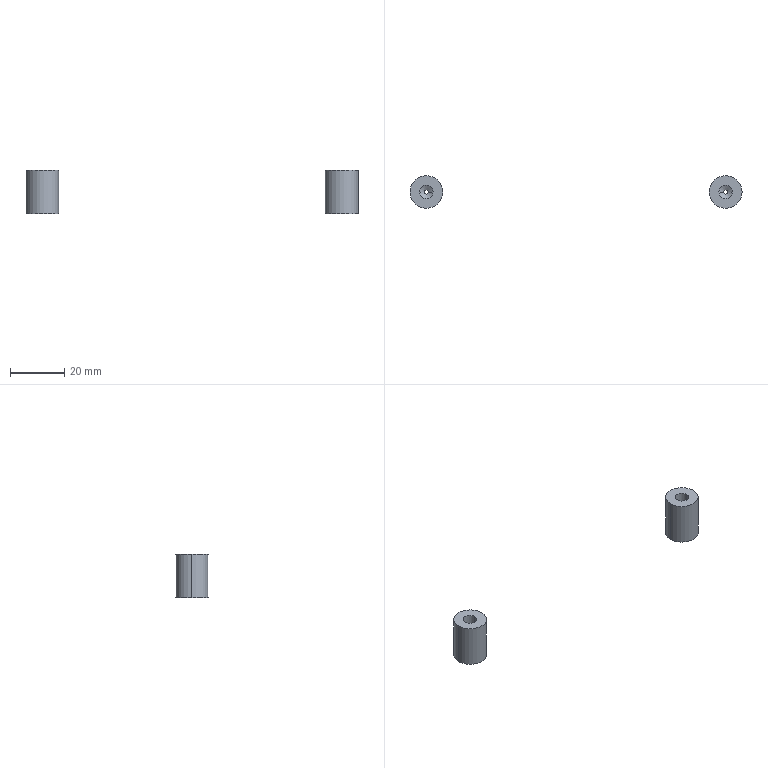Part | SolidWorks | features BaseBody 2 | 2 solids | 16 faces | box 122 x 12 x 16 mm | volume 3011 mm3 | cylinder 8 | cone 4 | plane 4 | commonest cylinder face diameters 5 x4 12 x4
STEP:
#1=CARTESIAN_POINT('',(-6.,0.,16.));
#2=VERTEX_POINT('',#1);
#3=CARTESIAN_POINT('',(6.,0.,16.));
#4=VERTEX_POINT('',#3);
#5=CARTESIAN_POINT('',(0.,0.,16.));
#6=DIRECTION('',(0.,0.,-1.));
#7=DIRECTION('',(-1.,0.,0.));
#8=AXIS2_PLACEMENT_3D('',#5,#6,#7);
#9=CIRCLE('',#8,6.);
#10=EDGE_CURVE('',#2,#4,#9,.T.);
#11=ORIENTED_EDGE('',*,*,#10,.T.);
#12=CARTESIAN_POINT('',(6.,0.,0.));
#13=VERTEX_POINT('',#12);
#14=CARTESIAN_POINT('',(6.,0.,16.));
#15=DIRECTION('',(0.,0.,-1.));
#16=VECTOR('',#15,1000.);
#17=LINE('',#14,#16);
#18=EDGE_CURVE('',#4,#13,#17,.T.);
#19=ORIENTED_EDGE('',*,*,#18,.T.);
#20=CARTESIAN_POINT('',(-6.,0.,0.));
#21=VERTEX_POINT('',#20);
#22=CARTESIAN_POINT('',(0.,0.,0.));
#23=DIRECTION('',(0.,0.,1.));
#24=DIRECTION('',(-1.,0.,0.));
#25=AXIS2_PLACEMENT_3D('',#22,#23,#24);
#26=CIRCLE('',#25,6.);
#27=EDGE_CURVE('',#13,#21,#26,.T.);
#28=ORIENTED_EDGE('',*,*,#27,.T.);
#29=CARTESIAN_POINT('',(-6.,0.,16.));
#30=DIRECTION('',(0.,0.,-1.));
#31=VECTOR('',#30,1000.);
#32=LINE('',#29,#31);
#33=EDGE_CURVE('',#2,#21,#32,.T.);
#34=ORIENTED_EDGE('',*,*,#33,.F.);
#35=EDGE_LOOP('',(#11,#19,#28,#34));
#36=FACE_OUTER_BOUND('',#35,.T.);
#37=CARTESIAN_POINT('',(0.,0.,16.));
#38=DIRECTION('',(0.,0.,-1.));
#39=DIRECTION('',(-1.,0.,0.));
#40=AXIS2_PLACEMENT_3D('',#37,#38,#39);
#41=CYLINDRICAL_SURFACE('',#40,6.);
#42=ADVANCED_FACE('',(#36),#41,.T.);
#43=CARTESIAN_POINT('',(0.8357,0.,0.));
#44=VERTEX_POINT('',#43);
#45=CARTESIAN_POINT('',(-0.8357,0.,0.));
#46=VERTEX_POINT('',#45);
#47=CARTESIAN_POINT('',(0.,0.,0.));
#48=DIRECTION('',(0.,0.,-1.));
#49=DIRECTION('',(1.,0.,0.));
#50=AXIS2_PLACEMENT_3D('',#47,#48,#49);
#51=CIRCLE('',#50,0.8357);
#52=EDGE_CURVE('',#44,#46,#51,.T.);
#53=ORIENTED_EDGE('',*,*,#52,.T.);
#54=CARTESIAN_POINT('',(-2.5,0.,1.));
#55=VERTEX_POINT('',#54);
#56=CARTESIAN_POINT('',(-2.5,0.,1.));
#57=DIRECTION('',(-0.8572,0.,0.515));
#58=VECTOR('',#57,1000.);
#59=LINE('',#56,#58);
#60=EDGE_CURVE('',#46,#55,#59,.T.);
#61=ORIENTED_EDGE('',*,*,#60,.T.);
#62=CARTESIAN_POINT('',(2.5,0.,1.));
#63=VERTEX_POINT('',#62);
#64=CARTESIAN_POINT('',(0.,0.,1.));
#65=DIRECTION('',(0.,0.,-1.));
#66=DIRECTION('',(1.,0.,0.));
#67=AXIS2_PLACEMENT_3D('',#64,#65,#66);
#68=CIRCLE('',#67,2.5);
#69=EDGE_CURVE('',#63,#55,#68,.T.);
#70=ORIENTED_EDGE('',*,*,#69,.F.);
#71=CARTESIAN_POINT('',(2.5,0.,1.));
#72=DIRECTION('',(0.8572,0.,0.515));
#73=VECTOR('',#72,1000.);
#74=LINE('',#71,#73);
#75=EDGE_CURVE('',#44,#63,#74,.T.);
#76=ORIENTED_EDGE('',*,*,#75,.F.);
#77=EDGE_LOOP('',(#53,#61,#70,#76));
#78=FACE_OUTER_BOUND('',#77,.T.);
#79=CARTESIAN_POINT('',(0.,0.,1.));
#80=DIRECTION('',(0.,0.,1.));
#81=DIRECTION('',(1.,0.,0.));
#82=AXIS2_PLACEMENT_3D('',#79,#80,#81);
#83=CONICAL_SURFACE('',#82,2.5,1.03);
#84=ADVANCED_FACE('',(#78),#83,.F.);
#85=ORIENTED_EDGE('',*,*,#69,.T.);
#86=CARTESIAN_POINT('',(-2.5,0.,16.));
#87=VERTEX_POINT('',#86);
#88=CARTESIAN_POINT('',(-2.5,0.,16.));
#89=DIRECTION('',(0.,0.,1.));
#90=VECTOR('',#89,1000.);
#91=LINE('',#88,#90);
#92=EDGE_CURVE('',#55,#87,#91,.T.);
#93=ORIENTED_EDGE('',*,*,#92,.T.);
#94=CARTESIAN_POINT('',(2.5,0.,16.));
#95=VERTEX_POINT('',#94);
#96=CARTESIAN_POINT('',(0.,0.,16.));
#97=DIRECTION('',(0.,0.,-1.));
#98=DIRECTION('',(1.,0.,0.));
#99=AXIS2_PLACEMENT_3D('',#96,#97,#98);
#100=CIRCLE('',#99,2.5);
#101=EDGE_CURVE('',#95,#87,#100,.T.);
#102=ORIENTED_EDGE('',*,*,#101,.F.);
#103=CARTESIAN_POINT('',(2.5,0.,16.));
#104=DIRECTION('',(0.,0.,1.));
#105=VECTOR('',#104,1000.);
#106=LINE('',#103,#105);
#107=EDGE_CURVE('',#63,#95,#106,.T.);
#108=ORIENTED_EDGE('',*,*,#107,.F.);
#109=EDGE_LOOP('',(#85,#93,#102,#108));
#110=FACE_OUTER_BOUND('',#109,.T.);
#111=CARTESIAN_POINT('',(0.,0.,16.));
#112=DIRECTION('',(0.,0.,1.));
#113=DIRECTION('',(1.,0.,0.));
#114=AXIS2_PLACEMENT_3D('',#111,#112,#113);
#115=CYLINDRICAL_SURFACE('',#114,2.5);
#116=ADVANCED_FACE('',(#110),#115,.F.);
#117=ORIENTED_EDGE('',*,*,#18,.F.);
#118=CARTESIAN_POINT('',(0.,0.,16.));
#119=DIRECTION('',(0.,0.,-1.));
#120=DIRECTION('',(-1.,0.,0.));
#121=AXIS2_PLACEMENT_3D('',#118,#119,#120);
#122=CIRCLE('',#121,6.);
#123=EDGE_CURVE('',#4,#2,#122,.T.);
#124=ORIENTED_EDGE('',*,*,#123,.T.);
#125=ORIENTED_EDGE('',*,*,#33,.T.);
#126=CARTESIAN_POINT('',(0.,0.,0.));
#127=DIRECTION('',(0.,0.,1.));
#128=DIRECTION('',(-1.,0.,0.));
#129=AXIS2_PLACEMENT_3D('',#126,#127,#128);
#130=CIRCLE('',#129,6.);
#131=EDGE_CURVE('',#21,#13,#130,.T.);
#132=ORIENTED_EDGE('',*,*,#131,.T.);
#133=EDGE_LOOP('',(#117,#124,#125,#132));
#134=FACE_OUTER_BOUND('',#133,.T.);
#135=CARTESIAN_POINT('',(0.,0.,16.));
#136=DIRECTION('',(0.,0.,-1.));
#137=DIRECTION('',(-1.,0.,0.));
#138=AXIS2_PLACEMENT_3D('',#135,#136,#137);
#139=CYLINDRICAL_SURFACE('',#138,6.);
#140=ADVANCED_FACE('',(#134),#139,.T.);
#141=ORIENTED_EDGE('',*,*,#131,.F.);
#142=ORIENTED_EDGE('',*,*,#27,.F.);
#143=EDGE_LOOP('',(#141,#142));
#144=FACE_OUTER_BOUND('',#143,.T.);
#145=ORIENTED_EDGE('',*,*,#52,.F.);
#146=CARTESIAN_POINT('',(0.,0.,0.));
#147=DIRECTION('',(0.,0.,-1.));
#148=DIRECTION('',(1.,0.,0.));
#149=AXIS2_PLACEMENT_3D('',#146,#147,#148);
#150=CIRCLE('',#149,0.8357);
#151=EDGE_CURVE('',#46,#44,#150,.T.);
#152=ORIENTED_EDGE('',*,*,#151,.F.);
#153=EDGE_LOOP('',(#145,#152));
#154=FACE_BOUND('',#153,.T.);
#155=CARTESIAN_POINT('',(0.,0.,0.));
#156=DIRECTION('',(0.,0.,1.));
#157=DIRECTION('',(1.,0.,0.));
#158=AXIS2_PLACEMENT_3D('',#155,#156,#157);
#159=PLANE('',#158);
#160=ADVANCED_FACE('',(#144,#154),#159,.F.);
#161=ORIENTED_EDGE('',*,*,#10,.F.);
#162=ORIENTED_EDGE('',*,*,#123,.F.);
#163=EDGE_LOOP('',(#161,#162));
#164=FACE_OUTER_BOUND('',#163,.T.);
#165=ORIENTED_EDGE('',*,*,#101,.T.);
#166=CARTESIAN_POINT('',(0.,0.,16.));
#167=DIRECTION('',(0.,0.,-1.));
#168=DIRECTION('',(1.,0.,0.));
#169=AXIS2_PLACEMENT_3D('',#166,#167,#168);
#170=CIRCLE('',#169,2.5);
#171=EDGE_CURVE('',#87,#95,#170,.T.);
#172=ORIENTED_EDGE('',*,*,#171,.T.);
#173=EDGE_LOOP('',(#165,#172));
#174=FACE_BOUND('',#173,.T.);
#175=CARTESIAN_POINT('',(0.,0.,16.));
#176=DIRECTION('',(0.,0.,1.));
#177=DIRECTION('',(1.,0.,0.));
#178=AXIS2_PLACEMENT_3D('',#175,#176,#177);
#179=PLANE('',#178);
#180=ADVANCED_FACE('',(#164,#174),#179,.T.);
#181=ORIENTED_EDGE('',*,*,#60,.F.);
#182=ORIENTED_EDGE('',*,*,#151,.T.);
#183=ORIENTED_EDGE('',*,*,#75,.T.);
#184=CARTESIAN_POINT('',(0.,0.,1.));
#185=DIRECTION('',(0.,0.,-1.));
#186=DIRECTION('',(1.,0.,0.));
#187=AXIS2_PLACEMENT_3D('',#184,#185,#186);
#188=CIRCLE('',#187,2.5);
#189=EDGE_CURVE('',#55,#63,#188,.T.);
#190=ORIENTED_EDGE('',*,*,#189,.F.);
#191=EDGE_LOOP('',(#181,#182,#183,#190));
#192=FACE_OUTER_BOUND('',#191,.T.);
#193=CARTESIAN_POINT('',(0.,0.,1.));
#194=DIRECTION('',(0.,0.,1.));
#195=DIRECTION('',(1.,0.,0.));
#196=AXIS2_PLACEMENT_3D('',#193,#194,#195);
#197=CONICAL_SURFACE('',#196,2.5,1.03);
#198=ADVANCED_FACE('',(#192),#197,.F.);
#199=ORIENTED_EDGE('',*,*,#92,.F.);
#200=ORIENTED_EDGE('',*,*,#189,.T.);
#201=ORIENTED_EDGE('',*,*,#107,.T.);
#202=ORIENTED_EDGE('',*,*,#171,.F.);
#203=EDGE_LOOP('',(#199,#200,#201,#202));
#204=FACE_OUTER_BOUND('',#203,.T.);
#205=CARTESIAN_POINT('',(0.,0.,16.));
#206=DIRECTION('',(0.,0.,1.));
#207=DIRECTION('',(1.,0.,0.));
#208=AXIS2_PLACEMENT_3D('',#205,#206,#207);
#209=CYLINDRICAL_SURFACE('',#208,2.5);
#210=ADVANCED_FACE('',(#204),#209,.F.);
#211=CLOSED_SHELL('',(#42,#84,#116,#140,#160,#180,#198,#210));
#212=MANIFOLD_SOLID_BREP('',#211);
#213=CARTESIAN_POINT('',(104.,0.,16.));
#214=VERTEX_POINT('',#213);
#215=CARTESIAN_POINT('',(116.,0.,16.));
#216=VERTEX_POINT('',#215);
#217=CARTESIAN_POINT('',(110.,0.,16.));
#218=DIRECTION('',(0.,0.,-1.));
#219=DIRECTION('',(-1.,0.,0.));
#220=AXIS2_PLACEMENT_3D('',#217,#218,#219);
#221=CIRCLE('',#220,6.);
#222=EDGE_CURVE('',#214,#216,#221,.T.);
#223=ORIENTED_EDGE('',*,*,#222,.T.);
#224=CARTESIAN_POINT('',(116.,0.,0.));
#225=VERTEX_POINT('',#224);
#226=CARTESIAN_POINT('',(116.,0.,16.));
#227=DIRECTION('',(0.,0.,-1.));
#228=VECTOR('',#227,1000.);
#229=LINE('',#226,#228);
#230=EDGE_CURVE('',#216,#225,#229,.T.);
#231=ORIENTED_EDGE('',*,*,#230,.T.);
#232=CARTESIAN_POINT('',(104.,0.,0.));
#233=VERTEX_POINT('',#232);
#234=CARTESIAN_POINT('',(110.,0.,0.));
#235=DIRECTION('',(0.,0.,1.));
#236=DIRECTION('',(-1.,0.,0.));
#237=AXIS2_PLACEMENT_3D('',#234,#235,#236);
#238=CIRCLE('',#237,6.);
#239=EDGE_CURVE('',#225,#233,#238,.T.);
#240=ORIENTED_EDGE('',*,*,#239,.T.);
#241=CARTESIAN_POINT('',(104.,0.,16.));
#242=DIRECTION('',(0.,0.,-1.));
#243=VECTOR('',#242,1000.);
#244=LINE('',#241,#243);
#245=EDGE_CURVE('',#214,#233,#244,.T.);
#246=ORIENTED_EDGE('',*,*,#245,.F.);
#247=EDGE_LOOP('',(#223,#231,#240,#246));
#248=FACE_OUTER_BOUND('',#247,.T.);
#249=CARTESIAN_POINT('',(110.,0.,16.));
#250=DIRECTION('',(0.,0.,-1.));
#251=DIRECTION('',(-1.,0.,0.));
#252=AXIS2_PLACEMENT_3D('',#249,#250,#251);
#253=CYLINDRICAL_SURFACE('',#252,6.);
#254=ADVANCED_FACE('',(#248),#253,.T.);
#255=CARTESIAN_POINT('',(110.836,0.,0.));
#256=VERTEX_POINT('',#255);
#257=CARTESIAN_POINT('',(109.164,0.,0.));
#258=VERTEX_POINT('',#257);
#259=CARTESIAN_POINT('',(110.,0.,0.));
#260=DIRECTION('',(0.,0.,-1.));
#261=DIRECTION('',(1.,0.,0.));
#262=AXIS2_PLACEMENT_3D('',#259,#260,#261);
#263=CIRCLE('',#262,0.8357);
#264=EDGE_CURVE('',#256,#258,#263,.T.);
#265=ORIENTED_EDGE('',*,*,#264,.T.);
#266=CARTESIAN_POINT('',(107.5,0.,1.));
#267=VERTEX_POINT('',#266);
#268=CARTESIAN_POINT('',(107.5,0.,1.));
#269=DIRECTION('',(-0.8572,0.,0.515));
#270=VECTOR('',#269,1000.);
#271=LINE('',#268,#270);
#272=EDGE_CURVE('',#258,#267,#271,.T.);
#273=ORIENTED_EDGE('',*,*,#272,.T.);
#274=CARTESIAN_POINT('',(112.5,0.,1.));
#275=VERTEX_POINT('',#274);
#276=CARTESIAN_POINT('',(110.,0.,1.));
#277=DIRECTION('',(0.,0.,-1.));
#278=DIRECTION('',(1.,0.,0.));
#279=AXIS2_PLACEMENT_3D('',#276,#277,#278);
#280=CIRCLE('',#279,2.5);
#281=EDGE_CURVE('',#275,#267,#280,.T.);
#282=ORIENTED_EDGE('',*,*,#281,.F.);
#283=CARTESIAN_POINT('',(112.5,0.,1.));
#284=DIRECTION('',(0.8572,0.,0.515));
#285=VECTOR('',#284,1000.);
#286=LINE('',#283,#285);
#287=EDGE_CURVE('',#256,#275,#286,.T.);
#288=ORIENTED_EDGE('',*,*,#287,.F.);
#289=EDGE_LOOP('',(#265,#273,#282,#288));
#290=FACE_OUTER_BOUND('',#289,.T.);
#291=CARTESIAN_POINT('',(110.,0.,1.));
#292=DIRECTION('',(0.,0.,1.));
#293=DIRECTION('',(1.,0.,0.));
#294=AXIS2_PLACEMENT_3D('',#291,#292,#293);
#295=CONICAL_SURFACE('',#294,2.5,1.03);
#296=ADVANCED_FACE('',(#290),#295,.F.);
#297=ORIENTED_EDGE('',*,*,#281,.T.);
#298=CARTESIAN_POINT('',(107.5,0.,16.));
#299=VERTEX_POINT('',#298);
#300=CARTESIAN_POINT('',(107.5,0.,16.));
#301=DIRECTION('',(0.,0.,1.));
#302=VECTOR('',#301,1000.);
#303=LINE('',#300,#302);
#304=EDGE_CURVE('',#267,#299,#303,.T.);
#305=ORIENTED_EDGE('',*,*,#304,.T.);
#306=CARTESIAN_POINT('',(112.5,0.,16.));
#307=VERTEX_POINT('',#306);
#308=CARTESIAN_POINT('',(110.,0.,16.));
#309=DIRECTION('',(0.,0.,-1.));
#310=DIRECTION('',(1.,0.,0.));
#311=AXIS2_PLACEMENT_3D('',#308,#309,#310);
#312=CIRCLE('',#311,2.5);
#313=EDGE_CURVE('',#307,#299,#312,.T.);
#314=ORIENTED_EDGE('',*,*,#313,.F.);
#315=CARTESIAN_POINT('',(112.5,0.,16.));
#316=DIRECTION('',(0.,0.,1.));
#317=VECTOR('',#316,1000.);
#318=LINE('',#315,#317);
#319=EDGE_CURVE('',#275,#307,#318,.T.);
#320=ORIENTED_EDGE('',*,*,#319,.F.);
#321=EDGE_LOOP('',(#297,#305,#314,#320));
#322=FACE_OUTER_BOUND('',#321,.T.);
#323=CARTESIAN_POINT('',(110.,0.,16.));
#324=DIRECTION('',(0.,0.,1.));
#325=DIRECTION('',(1.,0.,0.));
#326=AXIS2_PLACEMENT_3D('',#323,#324,#325);
#327=CYLINDRICAL_SURFACE('',#326,2.5);
#328=ADVANCED_FACE('',(#322),#327,.F.);
#329=ORIENTED_EDGE('',*,*,#230,.F.);
#330=CARTESIAN_POINT('',(110.,0.,16.));
#331=DIRECTION('',(0.,0.,-1.));
#332=DIRECTION('',(-1.,0.,0.));
#333=AXIS2_PLACEMENT_3D('',#330,#331,#332);
#334=CIRCLE('',#333,6.);
#335=EDGE_CURVE('',#216,#214,#334,.T.);
#336=ORIENTED_EDGE('',*,*,#335,.T.);
#337=ORIENTED_EDGE('',*,*,#245,.T.);
#338=CARTESIAN_POINT('',(110.,0.,0.));
#339=DIRECTION('',(0.,0.,1.));
#340=DIRECTION('',(-1.,0.,0.));
#341=AXIS2_PLACEMENT_3D('',#338,#339,#340);
#342=CIRCLE('',#341,6.);
#343=EDGE_CURVE('',#233,#225,#342,.T.);
#344=ORIENTED_EDGE('',*,*,#343,.T.);
#345=EDGE_LOOP('',(#329,#336,#337,#344));
#346=FACE_OUTER_BOUND('',#345,.T.);
#347=CARTESIAN_POINT('',(110.,0.,16.));
#348=DIRECTION('',(0.,0.,-1.));
#349=DIRECTION('',(-1.,0.,0.));
#350=AXIS2_PLACEMENT_3D('',#347,#348,#349);
#351=CYLINDRICAL_SURFACE('',#350,6.);
#352=ADVANCED_FACE('',(#346),#351,.T.);
#353=ORIENTED_EDGE('',*,*,#343,.F.);
#354=ORIENTED_EDGE('',*,*,#239,.F.);
#355=EDGE_LOOP('',(#353,#354));
#356=FACE_OUTER_BOUND('',#355,.T.);
#357=ORIENTED_EDGE('',*,*,#264,.F.);
#358=CARTESIAN_POINT('',(110.,0.,0.));
#359=DIRECTION('',(0.,0.,-1.));
#360=DIRECTION('',(1.,0.,0.));
#361=AXIS2_PLACEMENT_3D('',#358,#359,#360);
#362=CIRCLE('',#361,0.8357);
#363=EDGE_CURVE('',#258,#256,#362,.T.);
#364=ORIENTED_EDGE('',*,*,#363,.F.);
#365=EDGE_LOOP('',(#357,#364));
#366=FACE_BOUND('',#365,.T.);
#367=CARTESIAN_POINT('',(110.,0.,0.));
#368=DIRECTION('',(0.,0.,1.));
#369=DIRECTION('',(1.,0.,0.));
#370=AXIS2_PLACEMENT_3D('',#367,#368,#369);
#371=PLANE('',#370);
#372=ADVANCED_FACE('',(#356,#366),#371,.F.);
#373=ORIENTED_EDGE('',*,*,#222,.F.);
#374=ORIENTED_EDGE('',*,*,#335,.F.);
#375=EDGE_LOOP('',(#373,#374));
#376=FACE_OUTER_BOUND('',#375,.T.);
#377=ORIENTED_EDGE('',*,*,#313,.T.);
#378=CARTESIAN_POINT('',(110.,0.,16.));
#379=DIRECTION('',(0.,0.,-1.));
#380=DIRECTION('',(1.,0.,0.));
#381=AXIS2_PLACEMENT_3D('',#378,#379,#380);
#382=CIRCLE('',#381,2.5);
#383=EDGE_CURVE('',#299,#307,#382,.T.);
#384=ORIENTED_EDGE('',*,*,#383,.T.);
#385=EDGE_LOOP('',(#377,#384));
#386=FACE_BOUND('',#385,.T.);
#387=CARTESIAN_POINT('',(110.,0.,16.));
#388=DIRECTION('',(0.,0.,1.));
#389=DIRECTION('',(1.,0.,0.));
#390=AXIS2_PLACEMENT_3D('',#387,#388,#389);
#391=PLANE('',#390);
#392=ADVANCED_FACE('',(#376,#386),#391,.T.);
#393=ORIENTED_EDGE('',*,*,#272,.F.);
#394=ORIENTED_EDGE('',*,*,#363,.T.);
#395=ORIENTED_EDGE('',*,*,#287,.T.);
#396=CARTESIAN_POINT('',(110.,0.,1.));
#397=DIRECTION('',(0.,0.,-1.));
#398=DIRECTION('',(1.,0.,0.));
#399=AXIS2_PLACEMENT_3D('',#396,#397,#398);
#400=CIRCLE('',#399,2.5);
#401=EDGE_CURVE('',#267,#275,#400,.T.);
#402=ORIENTED_EDGE('',*,*,#401,.F.);
#403=EDGE_LOOP('',(#393,#394,#395,#402));
#404=FACE_OUTER_BOUND('',#403,.T.);
#405=CARTESIAN_POINT('',(110.,0.,1.));
#406=DIRECTION('',(0.,0.,1.));
#407=DIRECTION('',(1.,0.,0.));
#408=AXIS2_PLACEMENT_3D('',#405,#406,#407);
#409=CONICAL_SURFACE('',#408,2.5,1.03);
#410=ADVANCED_FACE('',(#404),#409,.F.);
#411=ORIENTED_EDGE('',*,*,#304,.F.);
#412=ORIENTED_EDGE('',*,*,#401,.T.);
#413=ORIENTED_EDGE('',*,*,#319,.T.);
#414=ORIENTED_EDGE('',*,*,#383,.F.);
#415=EDGE_LOOP('',(#411,#412,#413,#414));
#416=FACE_OUTER_BOUND('',#415,.T.);
#417=CARTESIAN_POINT('',(110.,0.,16.));
#418=DIRECTION('',(0.,0.,1.));
#419=DIRECTION('',(1.,0.,0.));
#420=AXIS2_PLACEMENT_3D('',#417,#418,#419);
#421=CYLINDRICAL_SURFACE('',#420,2.5);
#422=ADVANCED_FACE('',(#416),#421,.F.);
#423=CLOSED_SHELL('',(#254,#296,#328,#352,#372,#392,#410,#422));
#424=MANIFOLD_SOLID_BREP('',#423);
#425=CARTESIAN_POINT('',(0.,0.,0.));
#426=DIRECTION('',(0.,0.,1.));
#427=DIRECTION('',(1.,0.,0.));
#428=AXIS2_PLACEMENT_3D('',#425,#426,#427);
#429=(LENGTH_UNIT()NAMED_UNIT(*)SI_UNIT(.MILLI.,.METRE.));
#430=UNCERTAINTY_MEASURE_WITH_UNIT(LENGTH_MEASURE(0.00001),#429,'','');
#431=(NAMED_UNIT(*)PLANE_ANGLE_UNIT()SI_UNIT($,.RADIAN.));
#432=(NAMED_UNIT(*)SI_UNIT($,.STERADIAN.)SOLID_ANGLE_UNIT());
#433=(GEOMETRIC_REPRESENTATION_CONTEXT(3)GLOBAL_UNCERTAINTY_ASSIGNED_CONTEXT((#430))GLOBAL_UNIT_ASSIGNED_CONTEXT((#429,#431,#432))REPRESENTATION_CONTEXT('',''));
#434=ADVANCED_BREP_SHAPE_REPRESENTATION('',(#212,#424,#428),#433);